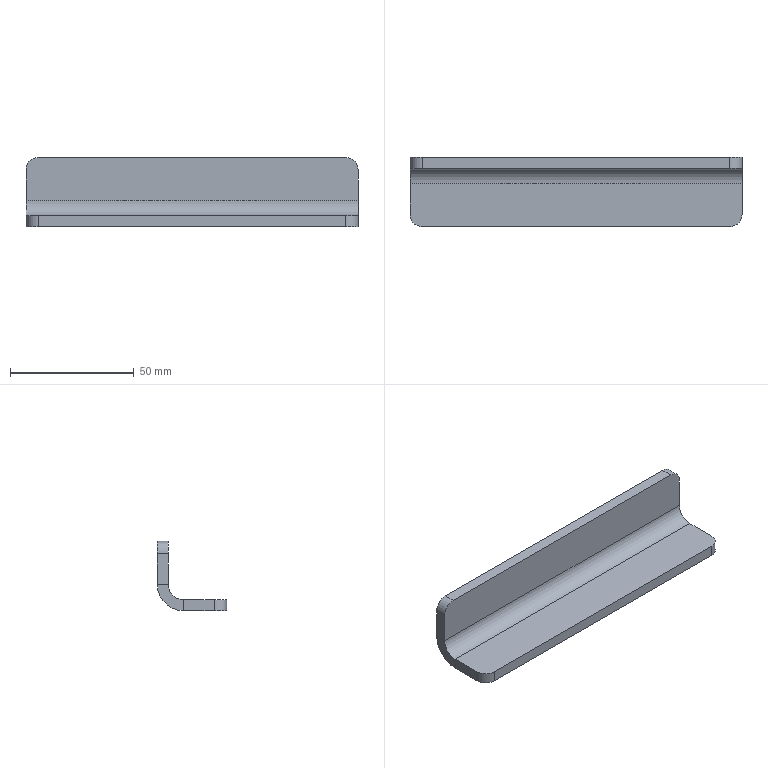Part | SolidWorks | features Fillet 1, FlatPattern 1, SMBaseFlange 1, SheetMetal 1 | 1 solid | 18 faces | box 134 x 28 x 28 mm | volume 28823 mm3 | plane 12 | cylinder 6 | commonest cylinder face diameters 10 x4 12 x1 21 x1
STEP:
#1=CARTESIAN_POINT('',(67.,-10.5,-28.));
#2=VERTEX_POINT('',#1);
#3=CARTESIAN_POINT('',(67.,-10.5,-23.5));
#4=VERTEX_POINT('',#3);
#5=CARTESIAN_POINT('',(67.,-10.5,-28.));
#6=DIRECTION('',(0.,0.,1.));
#7=VECTOR('',#6,1000.);
#8=LINE('',#5,#7);
#9=EDGE_CURVE('',#2,#4,#8,.T.);
#10=ORIENTED_EDGE('',*,*,#9,.F.);
#11=CARTESIAN_POINT('',(67.,0.,-17.5));
#12=VERTEX_POINT('',#11);
#13=CARTESIAN_POINT('',(67.,-10.5,-17.5));
#14=DIRECTION('',(-1.,0.,0.));
#15=DIRECTION('',(0.,0.,-1.));
#16=AXIS2_PLACEMENT_3D('',#13,#14,#15);
#17=CIRCLE('',#16,10.5);
#18=EDGE_CURVE('',#12,#2,#17,.T.);
#19=ORIENTED_EDGE('',*,*,#18,.F.);
#20=CARTESIAN_POINT('',(67.,-4.5,-17.5));
#21=VERTEX_POINT('',#20);
#22=CARTESIAN_POINT('',(67.,-4.5,-17.5));
#23=DIRECTION('',(0.,1.,0.));
#24=VECTOR('',#23,1000.);
#25=LINE('',#22,#24);
#26=EDGE_CURVE('',#21,#12,#25,.T.);
#27=ORIENTED_EDGE('',*,*,#26,.F.);
#28=CARTESIAN_POINT('',(67.,-10.5,-17.5));
#29=DIRECTION('',(-1.,0.,0.));
#30=DIRECTION('',(0.,0.,-1.));
#31=AXIS2_PLACEMENT_3D('',#28,#29,#30);
#32=CIRCLE('',#31,6.);
#33=EDGE_CURVE('',#21,#4,#32,.T.);
#34=ORIENTED_EDGE('',*,*,#33,.T.);
#35=EDGE_LOOP('',(#10,#19,#27,#34));
#36=FACE_OUTER_BOUND('',#35,.T.);
#37=CARTESIAN_POINT('',(67.,-10.5,-28.));
#38=DIRECTION('',(1.,0.,0.));
#39=DIRECTION('',(0.,0.,-1.));
#40=AXIS2_PLACEMENT_3D('',#37,#38,#39);
#41=PLANE('',#40);
#42=ADVANCED_FACE('',(#36),#41,.T.);
#43=CARTESIAN_POINT('',(67.,-23.,-23.5));
#44=VERTEX_POINT('',#43);
#45=CARTESIAN_POINT('',(67.,0.,-23.5));
#46=DIRECTION('',(0.,-1.,0.));
#47=VECTOR('',#46,1000.);
#48=LINE('',#45,#47);
#49=EDGE_CURVE('',#4,#44,#48,.T.);
#50=ORIENTED_EDGE('',*,*,#49,.T.);
#51=CARTESIAN_POINT('',(67.,-23.,-28.));
#52=VERTEX_POINT('',#51);
#53=CARTESIAN_POINT('',(67.,-23.,-17.5));
#54=DIRECTION('',(0.,0.,-1.));
#55=VECTOR('',#54,1000.);
#56=LINE('',#53,#55);
#57=EDGE_CURVE('',#44,#52,#56,.T.);
#58=ORIENTED_EDGE('',*,*,#57,.T.);
#59=CARTESIAN_POINT('',(67.,0.,-28.));
#60=DIRECTION('',(0.,-1.,0.));
#61=VECTOR('',#60,1000.);
#62=LINE('',#59,#61);
#63=EDGE_CURVE('',#2,#52,#62,.T.);
#64=ORIENTED_EDGE('',*,*,#63,.F.);
#65=ORIENTED_EDGE('',*,*,#9,.T.);
#66=EDGE_LOOP('',(#50,#58,#64,#65));
#67=FACE_OUTER_BOUND('',#66,.T.);
#68=CARTESIAN_POINT('',(67.,-4.5,-17.5));
#69=DIRECTION('',(1.,0.,0.));
#70=DIRECTION('',(0.,0.,-1.));
#71=AXIS2_PLACEMENT_3D('',#68,#69,#70);
#72=PLANE('',#71);
#73=ADVANCED_FACE('',(#67),#72,.T.);
#74=CARTESIAN_POINT('',(-67.,0.,-17.5));
#75=VERTEX_POINT('',#74);
#76=CARTESIAN_POINT('',(-67.,-4.5,-17.5));
#77=VERTEX_POINT('',#76);
#78=CARTESIAN_POINT('',(-67.,0.,-17.5));
#79=DIRECTION('',(0.,-1.,0.));
#80=VECTOR('',#79,1000.);
#81=LINE('',#78,#80);
#82=EDGE_CURVE('',#75,#77,#81,.T.);
#83=ORIENTED_EDGE('',*,*,#82,.F.);
#84=CARTESIAN_POINT('',(-67.,-10.5,-28.));
#85=VERTEX_POINT('',#84);
#86=CARTESIAN_POINT('',(-67.,-10.5,-17.5));
#87=DIRECTION('',(-1.,0.,0.));
#88=DIRECTION('',(0.,0.,-1.));
#89=AXIS2_PLACEMENT_3D('',#86,#87,#88);
#90=CIRCLE('',#89,10.5);
#91=EDGE_CURVE('',#75,#85,#90,.T.);
#92=ORIENTED_EDGE('',*,*,#91,.T.);
#93=CARTESIAN_POINT('',(-67.,-10.5,-23.5));
#94=VERTEX_POINT('',#93);
#95=CARTESIAN_POINT('',(-67.,-10.5,-23.5));
#96=DIRECTION('',(0.,0.,-1.));
#97=VECTOR('',#96,1000.);
#98=LINE('',#95,#97);
#99=EDGE_CURVE('',#94,#85,#98,.T.);
#100=ORIENTED_EDGE('',*,*,#99,.F.);
#101=CARTESIAN_POINT('',(-67.,-10.5,-17.5));
#102=DIRECTION('',(-1.,0.,0.));
#103=DIRECTION('',(0.,0.,-1.));
#104=AXIS2_PLACEMENT_3D('',#101,#102,#103);
#105=CIRCLE('',#104,6.);
#106=EDGE_CURVE('',#77,#94,#105,.T.);
#107=ORIENTED_EDGE('',*,*,#106,.F.);
#108=EDGE_LOOP('',(#83,#92,#100,#107));
#109=FACE_OUTER_BOUND('',#108,.T.);
#110=CARTESIAN_POINT('',(-67.,0.,-17.5));
#111=DIRECTION('',(-1.,0.,0.));
#112=DIRECTION('',(0.,0.,1.));
#113=AXIS2_PLACEMENT_3D('',#110,#111,#112);
#114=PLANE('',#113);
#115=ADVANCED_FACE('',(#109),#114,.T.);
#116=CARTESIAN_POINT('',(-67.,-4.5,-5.));
#117=VERTEX_POINT('',#116);
#118=CARTESIAN_POINT('',(-67.,-4.5,0.));
#119=DIRECTION('',(0.,0.,-1.));
#120=VECTOR('',#119,1000.);
#121=LINE('',#118,#120);
#122=EDGE_CURVE('',#117,#77,#121,.T.);
#123=ORIENTED_EDGE('',*,*,#122,.F.);
#124=CARTESIAN_POINT('',(-67.,0.,-5.));
#125=VERTEX_POINT('',#124);
#126=CARTESIAN_POINT('',(-67.,-10.5,-5.));
#127=DIRECTION('',(0.,1.,0.));
#128=VECTOR('',#127,1000.);
#129=LINE('',#126,#128);
#130=EDGE_CURVE('',#117,#125,#129,.T.);
#131=ORIENTED_EDGE('',*,*,#130,.T.);
#132=CARTESIAN_POINT('',(-67.,0.,0.));
#133=DIRECTION('',(0.,0.,-1.));
#134=VECTOR('',#133,1000.);
#135=LINE('',#132,#134);
#136=EDGE_CURVE('',#125,#75,#135,.T.);
#137=ORIENTED_EDGE('',*,*,#136,.T.);
#138=ORIENTED_EDGE('',*,*,#82,.T.);
#139=EDGE_LOOP('',(#123,#131,#137,#138));
#140=FACE_OUTER_BOUND('',#139,.T.);
#141=CARTESIAN_POINT('',(-67.,-10.5,-23.5));
#142=DIRECTION('',(-1.,0.,0.));
#143=DIRECTION('',(0.,0.,1.));
#144=AXIS2_PLACEMENT_3D('',#141,#142,#143);
#145=PLANE('',#144);
#146=ADVANCED_FACE('',(#140),#145,.T.);
#147=CARTESIAN_POINT('',(62.,-28.,-23.5));
#148=VERTEX_POINT('',#147);
#149=CARTESIAN_POINT('',(-62.,-28.,-23.5));
#150=VERTEX_POINT('',#149);
#151=CARTESIAN_POINT('',(67.,-28.,-23.5));
#152=DIRECTION('',(-1.,0.,0.));
#153=VECTOR('',#152,1000.);
#154=LINE('',#151,#153);
#155=EDGE_CURVE('',#148,#150,#154,.T.);
#156=ORIENTED_EDGE('',*,*,#155,.F.);
#157=CARTESIAN_POINT('',(62.,-23.,-23.5));
#158=DIRECTION('',(0.,0.,1.));
#159=DIRECTION('',(-1.,0.,0.));
#160=AXIS2_PLACEMENT_3D('',#157,#158,#159);
#161=CIRCLE('',#160,5.);
#162=EDGE_CURVE('',#148,#44,#161,.T.);
#163=ORIENTED_EDGE('',*,*,#162,.T.);
#164=ORIENTED_EDGE('',*,*,#49,.F.);
#165=CARTESIAN_POINT('',(67.,-10.5,-23.5));
#166=DIRECTION('',(-1.,0.,0.));
#167=VECTOR('',#166,1000.);
#168=LINE('',#165,#167);
#169=EDGE_CURVE('',#4,#94,#168,.T.);
#170=ORIENTED_EDGE('',*,*,#169,.T.);
#171=CARTESIAN_POINT('',(-67.,-23.,-23.5));
#172=VERTEX_POINT('',#171);
#173=CARTESIAN_POINT('',(-67.,0.,-23.5));
#174=DIRECTION('',(0.,-1.,0.));
#175=VECTOR('',#174,1000.);
#176=LINE('',#173,#175);
#177=EDGE_CURVE('',#94,#172,#176,.T.);
#178=ORIENTED_EDGE('',*,*,#177,.T.);
#179=CARTESIAN_POINT('',(-62.,-23.,-23.5));
#180=DIRECTION('',(0.,0.,1.));
#181=DIRECTION('',(-1.,0.,0.));
#182=AXIS2_PLACEMENT_3D('',#179,#180,#181);
#183=CIRCLE('',#182,5.);
#184=EDGE_CURVE('',#172,#150,#183,.T.);
#185=ORIENTED_EDGE('',*,*,#184,.T.);
#186=EDGE_LOOP('',(#156,#163,#164,#170,#178,#185));
#187=FACE_OUTER_BOUND('',#186,.T.);
#188=CARTESIAN_POINT('',(67.,0.,-23.5));
#189=DIRECTION('',(0.,0.,-1.));
#190=DIRECTION('',(-1.,0.,0.));
#191=AXIS2_PLACEMENT_3D('',#188,#189,#190);
#192=PLANE('',#191);
#193=ADVANCED_FACE('',(#187),#192,.F.);
#194=CARTESIAN_POINT('',(62.,-28.,-28.));
#195=VERTEX_POINT('',#194);
#196=CARTESIAN_POINT('',(-62.,-28.,-28.));
#197=VERTEX_POINT('',#196);
#198=CARTESIAN_POINT('',(67.,-28.,-28.));
#199=DIRECTION('',(-1.,0.,0.));
#200=VECTOR('',#199,1000.);
#201=LINE('',#198,#200);
#202=EDGE_CURVE('',#195,#197,#201,.T.);
#203=ORIENTED_EDGE('',*,*,#202,.F.);
#204=CARTESIAN_POINT('',(62.,-28.,-28.));
#205=DIRECTION('',(0.,0.,1.));
#206=VECTOR('',#205,1000.);
#207=LINE('',#204,#206);
#208=EDGE_CURVE('',#195,#148,#207,.T.);
#209=ORIENTED_EDGE('',*,*,#208,.T.);
#210=ORIENTED_EDGE('',*,*,#155,.T.);
#211=CARTESIAN_POINT('',(-62.,-28.,-28.));
#212=DIRECTION('',(0.,0.,-1.));
#213=VECTOR('',#212,1000.);
#214=LINE('',#211,#213);
#215=EDGE_CURVE('',#150,#197,#214,.T.);
#216=ORIENTED_EDGE('',*,*,#215,.T.);
#217=EDGE_LOOP('',(#203,#209,#210,#216));
#218=FACE_OUTER_BOUND('',#217,.T.);
#219=CARTESIAN_POINT('',(67.,-28.,-28.));
#220=DIRECTION('',(0.,-1.,0.));
#221=DIRECTION('',(0.,0.,-1.));
#222=AXIS2_PLACEMENT_3D('',#219,#220,#221);
#223=PLANE('',#222);
#224=ADVANCED_FACE('',(#218),#223,.T.);
#225=ORIENTED_EDGE('',*,*,#63,.T.);
#226=CARTESIAN_POINT('',(62.,-23.,-28.));
#227=DIRECTION('',(0.,0.,-1.));
#228=DIRECTION('',(-1.,0.,0.));
#229=AXIS2_PLACEMENT_3D('',#226,#227,#228);
#230=CIRCLE('',#229,5.);
#231=EDGE_CURVE('',#52,#195,#230,.T.);
#232=ORIENTED_EDGE('',*,*,#231,.T.);
#233=ORIENTED_EDGE('',*,*,#202,.T.);
#234=CARTESIAN_POINT('',(-67.,-23.,-28.));
#235=VERTEX_POINT('',#234);
#236=CARTESIAN_POINT('',(-62.,-23.,-28.));
#237=DIRECTION('',(0.,0.,-1.));
#238=DIRECTION('',(-1.,0.,0.));
#239=AXIS2_PLACEMENT_3D('',#236,#237,#238);
#240=CIRCLE('',#239,5.);
#241=EDGE_CURVE('',#197,#235,#240,.T.);
#242=ORIENTED_EDGE('',*,*,#241,.T.);
#243=CARTESIAN_POINT('',(-67.,0.,-28.));
#244=DIRECTION('',(0.,-1.,0.));
#245=VECTOR('',#244,1000.);
#246=LINE('',#243,#245);
#247=EDGE_CURVE('',#85,#235,#246,.T.);
#248=ORIENTED_EDGE('',*,*,#247,.F.);
#249=CARTESIAN_POINT('',(67.,-10.5,-28.));
#250=DIRECTION('',(-1.,0.,0.));
#251=VECTOR('',#250,1000.);
#252=LINE('',#249,#251);
#253=EDGE_CURVE('',#2,#85,#252,.T.);
#254=ORIENTED_EDGE('',*,*,#253,.F.);
#255=EDGE_LOOP('',(#225,#232,#233,#242,#248,#254));
#256=FACE_OUTER_BOUND('',#255,.T.);
#257=CARTESIAN_POINT('',(67.,0.,-28.));
#258=DIRECTION('',(0.,0.,-1.));
#259=DIRECTION('',(-1.,0.,0.));
#260=AXIS2_PLACEMENT_3D('',#257,#258,#259);
#261=PLANE('',#260);
#262=ADVANCED_FACE('',(#256),#261,.T.);
#263=ORIENTED_EDGE('',*,*,#91,.F.);
#264=CARTESIAN_POINT('',(67.,0.,-17.5));
#265=DIRECTION('',(-1.,0.,0.));
#266=VECTOR('',#265,1000.);
#267=LINE('',#264,#266);
#268=EDGE_CURVE('',#12,#75,#267,.T.);
#269=ORIENTED_EDGE('',*,*,#268,.F.);
#270=ORIENTED_EDGE('',*,*,#18,.T.);
#271=ORIENTED_EDGE('',*,*,#253,.T.);
#272=EDGE_LOOP('',(#263,#269,#270,#271));
#273=FACE_OUTER_BOUND('',#272,.T.);
#274=CARTESIAN_POINT('',(67.,-10.5,-17.5));
#275=DIRECTION('',(-1.,0.,0.));
#276=DIRECTION('',(0.,0.,1.));
#277=AXIS2_PLACEMENT_3D('',#274,#275,#276);
#278=CYLINDRICAL_SURFACE('',#277,10.5);
#279=ADVANCED_FACE('',(#273),#278,.T.);
#280=CARTESIAN_POINT('',(62.,0.,0.));
#281=VERTEX_POINT('',#280);
#282=CARTESIAN_POINT('',(-62.,0.,0.));
#283=VERTEX_POINT('',#282);
#284=CARTESIAN_POINT('',(67.,0.,0.));
#285=DIRECTION('',(-1.,0.,0.));
#286=VECTOR('',#285,1000.);
#287=LINE('',#284,#286);
#288=EDGE_CURVE('',#281,#283,#287,.T.);
#289=ORIENTED_EDGE('',*,*,#288,.F.);
#290=CARTESIAN_POINT('',(67.,0.,-5.));
#291=VERTEX_POINT('',#290);
#292=CARTESIAN_POINT('',(62.,0.,-5.));
#293=DIRECTION('',(0.,1.,0.));
#294=DIRECTION('',(0.,0.,1.));
#295=AXIS2_PLACEMENT_3D('',#292,#293,#294);
#296=CIRCLE('',#295,5.);
#297=EDGE_CURVE('',#281,#291,#296,.T.);
#298=ORIENTED_EDGE('',*,*,#297,.T.);
#299=CARTESIAN_POINT('',(67.,0.,0.));
#300=DIRECTION('',(0.,0.,-1.));
#301=VECTOR('',#300,1000.);
#302=LINE('',#299,#301);
#303=EDGE_CURVE('',#291,#12,#302,.T.);
#304=ORIENTED_EDGE('',*,*,#303,.T.);
#305=ORIENTED_EDGE('',*,*,#268,.T.);
#306=ORIENTED_EDGE('',*,*,#136,.F.);
#307=CARTESIAN_POINT('',(-62.,0.,-5.));
#308=DIRECTION('',(0.,1.,0.));
#309=DIRECTION('',(0.,0.,1.));
#310=AXIS2_PLACEMENT_3D('',#307,#308,#309);
#311=CIRCLE('',#310,5.);
#312=EDGE_CURVE('',#125,#283,#311,.T.);
#313=ORIENTED_EDGE('',*,*,#312,.T.);
#314=EDGE_LOOP('',(#289,#298,#304,#305,#306,#313));
#315=FACE_OUTER_BOUND('',#314,.T.);
#316=CARTESIAN_POINT('',(67.,0.,0.));
#317=DIRECTION('',(0.,1.,0.));
#318=DIRECTION('',(0.,0.,1.));
#319=AXIS2_PLACEMENT_3D('',#316,#317,#318);
#320=PLANE('',#319);
#321=ADVANCED_FACE('',(#315),#320,.T.);
#322=CARTESIAN_POINT('',(62.,-4.5,0.));
#323=VERTEX_POINT('',#322);
#324=CARTESIAN_POINT('',(-62.,-4.5,0.));
#325=VERTEX_POINT('',#324);
#326=CARTESIAN_POINT('',(67.,-4.5,0.));
#327=DIRECTION('',(-1.,0.,0.));
#328=VECTOR('',#327,1000.);
#329=LINE('',#326,#328);
#330=EDGE_CURVE('',#323,#325,#329,.T.);
#331=ORIENTED_EDGE('',*,*,#330,.F.);
#332=CARTESIAN_POINT('',(62.,-4.5,0.));
#333=DIRECTION('',(0.,1.,0.));
#334=VECTOR('',#333,1000.);
#335=LINE('',#332,#334);
#336=EDGE_CURVE('',#323,#281,#335,.T.);
#337=ORIENTED_EDGE('',*,*,#336,.T.);
#338=ORIENTED_EDGE('',*,*,#288,.T.);
#339=CARTESIAN_POINT('',(-62.,-4.5,0.));
#340=DIRECTION('',(0.,-1.,0.));
#341=VECTOR('',#340,1000.);
#342=LINE('',#339,#341);
#343=EDGE_CURVE('',#283,#325,#342,.T.);
#344=ORIENTED_EDGE('',*,*,#343,.T.);
#345=EDGE_LOOP('',(#331,#337,#338,#344));
#346=FACE_OUTER_BOUND('',#345,.T.);
#347=CARTESIAN_POINT('',(67.,-4.5,0.));
#348=DIRECTION('',(0.,0.,1.));
#349=DIRECTION('',(1.,0.,0.));
#350=AXIS2_PLACEMENT_3D('',#347,#348,#349);
#351=PLANE('',#350);
#352=ADVANCED_FACE('',(#346),#351,.T.);
#353=CARTESIAN_POINT('',(67.,-4.5,-5.));
#354=VERTEX_POINT('',#353);
#355=CARTESIAN_POINT('',(67.,-4.5,0.));
#356=DIRECTION('',(0.,0.,-1.));
#357=VECTOR('',#356,1000.);
#358=LINE('',#355,#357);
#359=EDGE_CURVE('',#354,#21,#358,.T.);
#360=ORIENTED_EDGE('',*,*,#359,.F.);
#361=CARTESIAN_POINT('',(62.,-4.5,-5.));
#362=DIRECTION('',(0.,-1.,0.));
#363=DIRECTION('',(0.,0.,1.));
#364=AXIS2_PLACEMENT_3D('',#361,#362,#363);
#365=CIRCLE('',#364,5.);
#366=EDGE_CURVE('',#354,#323,#365,.T.);
#367=ORIENTED_EDGE('',*,*,#366,.T.);
#368=ORIENTED_EDGE('',*,*,#330,.T.);
#369=CARTESIAN_POINT('',(-62.,-4.5,-5.));
#370=DIRECTION('',(0.,-1.,0.));
#371=DIRECTION('',(0.,0.,1.));
#372=AXIS2_PLACEMENT_3D('',#369,#370,#371);
#373=CIRCLE('',#372,5.);
#374=EDGE_CURVE('',#325,#117,#373,.T.);
#375=ORIENTED_EDGE('',*,*,#374,.T.);
#376=ORIENTED_EDGE('',*,*,#122,.T.);
#377=CARTESIAN_POINT('',(67.,-4.5,-17.5));
#378=DIRECTION('',(-1.,0.,0.));
#379=VECTOR('',#378,1000.);
#380=LINE('',#377,#379);
#381=EDGE_CURVE('',#21,#77,#380,.T.);
#382=ORIENTED_EDGE('',*,*,#381,.F.);
#383=EDGE_LOOP('',(#360,#367,#368,#375,#376,#382));
#384=FACE_OUTER_BOUND('',#383,.T.);
#385=CARTESIAN_POINT('',(67.,-4.5,0.));
#386=DIRECTION('',(0.,1.,0.));
#387=DIRECTION('',(0.,0.,1.));
#388=AXIS2_PLACEMENT_3D('',#385,#386,#387);
#389=PLANE('',#388);
#390=ADVANCED_FACE('',(#384),#389,.F.);
#391=ORIENTED_EDGE('',*,*,#106,.T.);
#392=ORIENTED_EDGE('',*,*,#169,.F.);
#393=ORIENTED_EDGE('',*,*,#33,.F.);
#394=ORIENTED_EDGE('',*,*,#381,.T.);
#395=EDGE_LOOP('',(#391,#392,#393,#394));
#396=FACE_OUTER_BOUND('',#395,.T.);
#397=CARTESIAN_POINT('',(67.,-10.5,-17.5));
#398=DIRECTION('',(-1.,0.,0.));
#399=DIRECTION('',(0.,0.,1.));
#400=AXIS2_PLACEMENT_3D('',#397,#398,#399);
#401=CYLINDRICAL_SURFACE('',#400,6.);
#402=ADVANCED_FACE('',(#396),#401,.F.);
#403=ORIENTED_EDGE('',*,*,#303,.F.);
#404=CARTESIAN_POINT('',(67.,-10.5,-5.));
#405=DIRECTION('',(0.,-1.,0.));
#406=VECTOR('',#405,1000.);
#407=LINE('',#404,#406);
#408=EDGE_CURVE('',#291,#354,#407,.T.);
#409=ORIENTED_EDGE('',*,*,#408,.T.);
#410=ORIENTED_EDGE('',*,*,#359,.T.);
#411=ORIENTED_EDGE('',*,*,#26,.T.);
#412=EDGE_LOOP('',(#403,#409,#410,#411));
#413=FACE_OUTER_BOUND('',#412,.T.);
#414=CARTESIAN_POINT('',(67.,-10.5,-17.5));
#415=DIRECTION('',(1.,0.,0.));
#416=DIRECTION('',(0.,0.,-1.));
#417=AXIS2_PLACEMENT_3D('',#414,#415,#416);
#418=PLANE('',#417);
#419=ADVANCED_FACE('',(#413),#418,.T.);
#420=ORIENTED_EDGE('',*,*,#247,.T.);
#421=CARTESIAN_POINT('',(-67.,-23.,-23.5));
#422=DIRECTION('',(0.,0.,1.));
#423=VECTOR('',#422,1000.);
#424=LINE('',#421,#423);
#425=EDGE_CURVE('',#235,#172,#424,.T.);
#426=ORIENTED_EDGE('',*,*,#425,.T.);
#427=ORIENTED_EDGE('',*,*,#177,.F.);
#428=ORIENTED_EDGE('',*,*,#99,.T.);
#429=EDGE_LOOP('',(#420,#426,#427,#428));
#430=FACE_OUTER_BOUND('',#429,.T.);
#431=CARTESIAN_POINT('',(-67.,-10.5,-17.5));
#432=DIRECTION('',(1.,0.,0.));
#433=DIRECTION('',(0.,0.,-1.));
#434=AXIS2_PLACEMENT_3D('',#431,#432,#433);
#435=PLANE('',#434);
#436=ADVANCED_FACE('',(#430),#435,.F.);
#437=ORIENTED_EDGE('',*,*,#366,.F.);
#438=ORIENTED_EDGE('',*,*,#408,.F.);
#439=ORIENTED_EDGE('',*,*,#297,.F.);
#440=ORIENTED_EDGE('',*,*,#336,.F.);
#441=EDGE_LOOP('',(#437,#438,#439,#440));
#442=FACE_OUTER_BOUND('',#441,.T.);
#443=CARTESIAN_POINT('',(62.,-4.5,-5.));
#444=DIRECTION('',(0.,1.,0.));
#445=DIRECTION('',(0.,0.,1.));
#446=AXIS2_PLACEMENT_3D('',#443,#444,#445);
#447=CYLINDRICAL_SURFACE('',#446,5.);
#448=ADVANCED_FACE('',(#442),#447,.T.);
#449=ORIENTED_EDGE('',*,*,#231,.F.);
#450=ORIENTED_EDGE('',*,*,#57,.F.);
#451=ORIENTED_EDGE('',*,*,#162,.F.);
#452=ORIENTED_EDGE('',*,*,#208,.F.);
#453=EDGE_LOOP('',(#449,#450,#451,#452));
#454=FACE_OUTER_BOUND('',#453,.T.);
#455=CARTESIAN_POINT('',(62.,-23.,-28.));
#456=DIRECTION('',(0.,0.,1.));
#457=DIRECTION('',(1.,0.,0.));
#458=AXIS2_PLACEMENT_3D('',#455,#456,#457);
#459=CYLINDRICAL_SURFACE('',#458,5.);
#460=ADVANCED_FACE('',(#454),#459,.T.);
#461=ORIENTED_EDGE('',*,*,#241,.F.);
#462=ORIENTED_EDGE('',*,*,#215,.F.);
#463=ORIENTED_EDGE('',*,*,#184,.F.);
#464=ORIENTED_EDGE('',*,*,#425,.F.);
#465=EDGE_LOOP('',(#461,#462,#463,#464));
#466=FACE_OUTER_BOUND('',#465,.T.);
#467=CARTESIAN_POINT('',(-62.,-23.,-17.5));
#468=DIRECTION('',(0.,0.,-1.));
#469=DIRECTION('',(-1.,0.,0.));
#470=AXIS2_PLACEMENT_3D('',#467,#468,#469);
#471=CYLINDRICAL_SURFACE('',#470,5.);
#472=ADVANCED_FACE('',(#466),#471,.T.);
#473=ORIENTED_EDGE('',*,*,#374,.F.);
#474=ORIENTED_EDGE('',*,*,#343,.F.);
#475=ORIENTED_EDGE('',*,*,#312,.F.);
#476=ORIENTED_EDGE('',*,*,#130,.F.);
#477=EDGE_LOOP('',(#473,#474,#475,#476));
#478=FACE_OUTER_BOUND('',#477,.T.);
#479=CARTESIAN_POINT('',(-62.,-10.5,-5.));
#480=DIRECTION('',(0.,1.,0.));
#481=DIRECTION('',(0.,0.,1.));
#482=AXIS2_PLACEMENT_3D('',#479,#480,#481);
#483=CYLINDRICAL_SURFACE('',#482,5.);
#484=ADVANCED_FACE('',(#478),#483,.T.);
#485=CLOSED_SHELL('',(#42,#73,#115,#146,#193,#224,#262,#279,#321,#352,#390,#402,#419,#436,#448,#460,#472,#484));
#486=MANIFOLD_SOLID_BREP('',#485);
#487=CARTESIAN_POINT('',(0.,0.,0.));
#488=DIRECTION('',(0.,0.,1.));
#489=DIRECTION('',(1.,0.,0.));
#490=AXIS2_PLACEMENT_3D('',#487,#488,#489);
#491=(LENGTH_UNIT()NAMED_UNIT(*)SI_UNIT(.MILLI.,.METRE.));
#492=UNCERTAINTY_MEASURE_WITH_UNIT(LENGTH_MEASURE(0.00001),#491,'','');
#493=(NAMED_UNIT(*)PLANE_ANGLE_UNIT()SI_UNIT($,.RADIAN.));
#494=(NAMED_UNIT(*)SI_UNIT($,.STERADIAN.)SOLID_ANGLE_UNIT());
#495=(GEOMETRIC_REPRESENTATION_CONTEXT(3)GLOBAL_UNCERTAINTY_ASSIGNED_CONTEXT((#492))GLOBAL_UNIT_ASSIGNED_CONTEXT((#491,#493,#494))REPRESENTATION_CONTEXT('',''));
#496=ADVANCED_BREP_SHAPE_REPRESENTATION('',(#486,#490),#495);